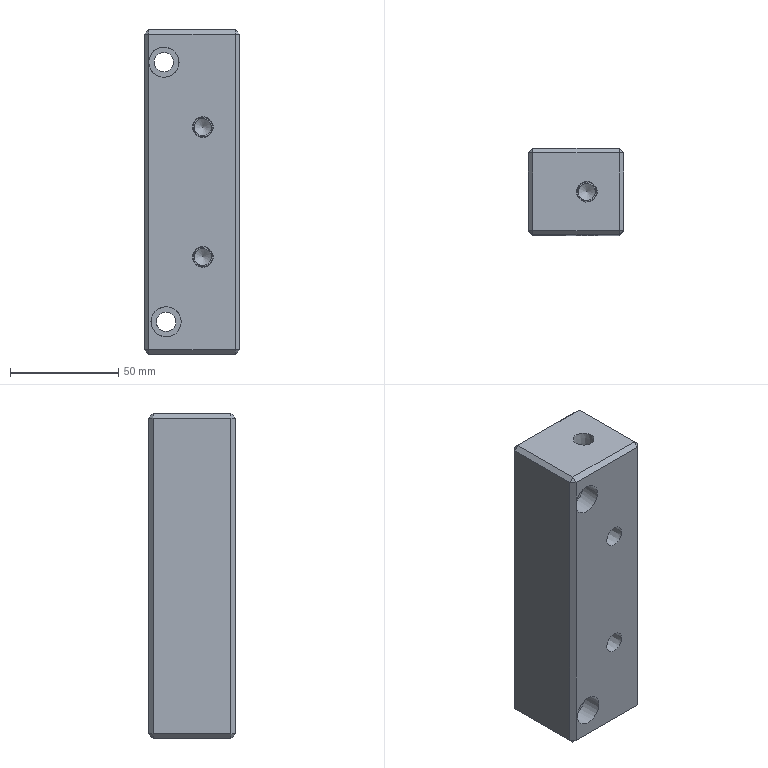Part | STEP file | 车灯-后视镜_id374_x_t | 1 solid | 76 faces | box 44 x 40 x 150 mm | volume 242093 mm3 | plane 36 | cylinder 24 | cone 16 | commonest cylinder face diameters 8 x20 9 x2 14 x2